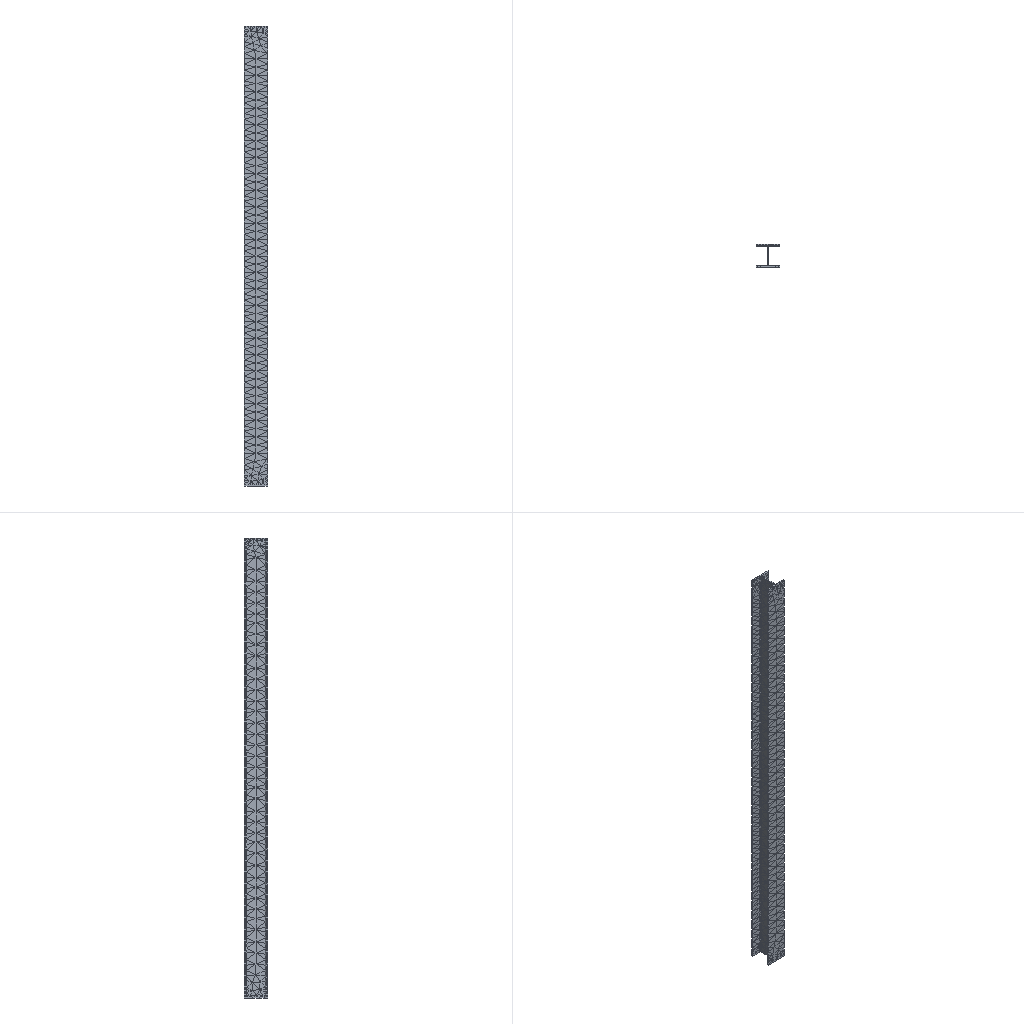Simulation study | ansys workbench
Set-up summary:
category,name,step,type,value,unit,region
solver,ansys_mapdl
solver,version,,,22.1
solver,version,,,22.1
units,MPA,,stated
analysis,deck1,,transient,transient
load_step,requested,,,2
analysis,nlgeom,,,True
mesh,nodes,,,10725
mesh,elements,,,5119
element_type,ANSYS 187 (type 1),,solid,5061
element_type,ANSYS 174 (type 2),,contact,58
element_type,ANSYS 170 (type 3),,target,0
load,load commands in deck,,count,3
bc,support commands in deck,,count,1
named_set,_FIXEDSU,,component
analysis,deck2,,static,static
load_step,requested,,,1
analysis,nlgeom,,,False
mesh,nodes,,,10725
mesh,elements,,,5119
element_type,ANSYS 187 (type 1),,solid,5061
element_type,ANSYS 174 (type 2),,contact,58
element_type,ANSYS 170 (type 3),,target,0
load,load commands in deck,,count,3
bc,support commands in deck,,count,1
named_set,_FIXEDSU,,component
material,1,,in results
material,1,,in results
check,setup vs results,,match,results also hold 0 node(s) and 1 element(s) the deck makes with ['EN']; those were not compared; 1 node(s) the solver created internally for pilot nodes (ansys-fenxi-2/H型钢有限元分析/H钢有限元分析_files/dp0/SYS-1/MECH/solve.out) are in the results only
check,setup vs results,,match,results also hold 0 node(s) and 1 element(s) the deck makes with ['EN']; those were not compared; 1 node(s) the solver created internally for pilot nodes (ansys-fenxi-2/H型钢有限元分析/H钢有限元分析_files/dp0/SYS/MECH/solve.out) are in the results only
Results summary:
result,analysis,,,static
result,last_loadstep,,,2
result,primary field,,,displacement
result,reaction total,2,FX,-0.01493,N
result,reaction total,2,FY,-0.001797,N
result,reaction total,2,FZ,-0.03615,N
result,mass,,,0.5595,"NMM: mm, ton, N, s, mV, mA, degC"
result,analysis,,,static
result,last_loadstep,,,1
result,primary field,,,displacement
result,reaction total,1,FX,4.9e-05,N
result,reaction total,1,FY,-0.000466,N
result,reaction total,1,FZ,-4e-06,N
result,mass,,,0.5595,"NMM: mm, ton, N, s, mV, mA, degC"